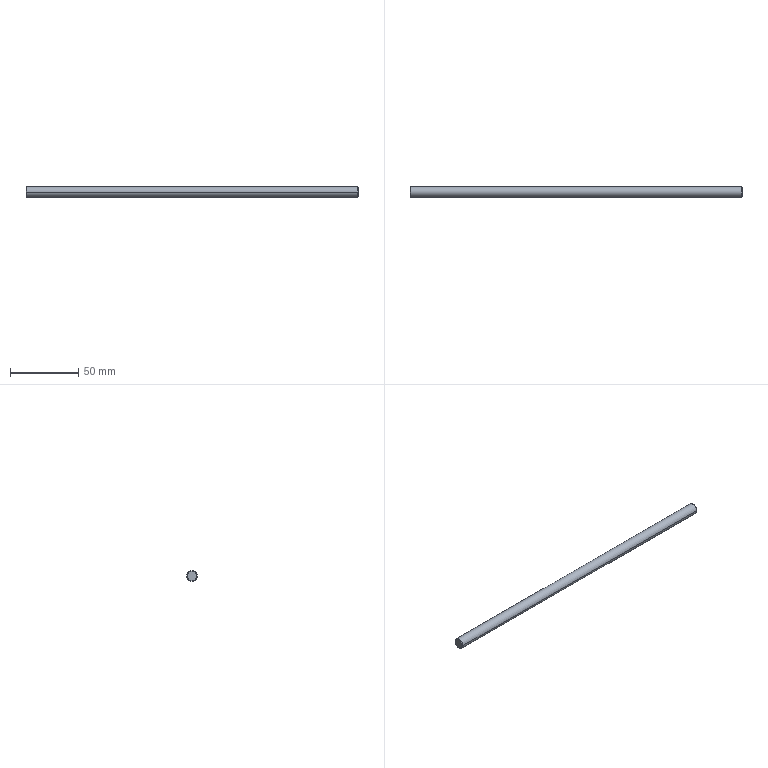Part | STEP file | 02-20 Φ8 polished rod | 1 solid | 8 faces | box 244 x 8 x 8 mm | volume 12259 mm3 | cone 4 | cylinder 2 | plane 2 | commonest cylinder face diameters 8 x2
STEP:
#1=CARTESIAN_POINT('',(0.,0.,0.));
#2=DIRECTION('',(0.,0.,1.));
#3=DIRECTION('',(1.,0.,0.));
#4=AXIS2_PLACEMENT_3D('',#1,#2,#3);
#5=CARTESIAN_POINT('',(-122.,0.,3.5));
#6=VERTEX_POINT('',#5);
#7=CARTESIAN_POINT('',(-122.,0.,-3.5));
#8=VERTEX_POINT('',#7);
#9=CARTESIAN_POINT('',(-122.,0.,0.));
#10=DIRECTION('',(-1.,0.,0.));
#11=DIRECTION('',(0.,0.,-1.));
#12=AXIS2_PLACEMENT_3D('',#9,#10,#11);
#13=CIRCLE('',#12,3.5);
#14=CARTESIAN_POINT('',(-122.,0.,0.));
#15=DIRECTION('',(1.,0.,0.));
#16=DIRECTION('',(0.,0.,-1.));
#17=AXIS2_PLACEMENT_3D('',#14,#15,#16);
#18=CONICAL_SURFACE('',#17,3.5,0.7854);
#19=CARTESIAN_POINT('',(6.283,0.));
#20=DIRECTION('',(-1.,0.));
#21=VECTOR('',#20,1.);
#22=LINE('',#19,#21);
#23=(GEOMETRIC_REPRESENTATION_CONTEXT(2)PARAMETRIC_REPRESENTATION_CONTEXT()REPRESENTATION_CONTEXT('',''));
#24=DEFINITIONAL_REPRESENTATION('',(#22),#23);
#25=PCURVE('',#18,#24);
#26=CARTESIAN_POINT('',(-122.,-3.542,3.542));
#27=DIRECTION('',(1.,0.,0.));
#28=DIRECTION('',(0.,0.,-1.));
#29=AXIS2_PLACEMENT_3D('',#26,#27,#28);
#30=PLANE('',#29);
#31=CARTESIAN_POINT('',(7.042,3.542));
#32=CARTESIAN_POINT('',(7.042,-2.52));
#33=CARTESIAN_POINT('',(1.792,0.5109));
#34=CARTESIAN_POINT('',(-3.458,3.542));
#35=CARTESIAN_POINT('',(1.792,6.573));
#36=CARTESIAN_POINT('',(7.042,9.604));
#37=CARTESIAN_POINT('',(7.042,3.542));
#38=(BOUNDED_CURVE()B_SPLINE_CURVE(2,(#31,#32,#33,#34,#35,#36,#37),.UNSPECIFIED.,.T.,.F.)B_SPLINE_CURVE_WITH_KNOTS((1,2,2,2,2,1),(-2.094,0.,2.094,4.189,6.283,8.378),.UNSPECIFIED.)CURVE()GEOMETRIC_REPRESENTATION_ITEM()RATIONAL_B_SPLINE_CURVE((1.,0.5,1.,0.5,1.,0.5,1.))REPRESENTATION_ITEM(''));
#39=(GEOMETRIC_REPRESENTATION_CONTEXT(2)PARAMETRIC_REPRESENTATION_CONTEXT()REPRESENTATION_CONTEXT('',''));
#40=DEFINITIONAL_REPRESENTATION('',(#38),#39);
#41=PCURVE('',#30,#40);
#42=SURFACE_CURVE('',#13,(#25,#41),.PCURVE_S1.);
#43=EDGE_CURVE('',#6,#8,#42,.T.);
#44=ORIENTED_EDGE('',*,*,#43,.F.);
#45=CARTESIAN_POINT('',(-121.5,0.,4.));
#46=VERTEX_POINT('',#45);
#47=CARTESIAN_POINT('',(-122.,0.,3.5));
#48=DIRECTION('',(0.7071,0.,0.7071));
#49=VECTOR('',#48,1.);
#50=LINE('',#47,#49);
#51=CARTESIAN_POINT('',(3.142,0.));
#52=DIRECTION('',(0.,1.));
#53=VECTOR('',#52,1.);
#54=LINE('',#51,#53);
#55=(GEOMETRIC_REPRESENTATION_CONTEXT(2)PARAMETRIC_REPRESENTATION_CONTEXT()REPRESENTATION_CONTEXT('',''));
#56=DEFINITIONAL_REPRESENTATION('',(#54),#55);
#57=PCURVE('',#18,#56);
#58=CARTESIAN_POINT('',(-122.,0.,0.));
#59=DIRECTION('',(1.,0.,0.));
#60=DIRECTION('',(0.,0.,-1.));
#61=AXIS2_PLACEMENT_3D('',#58,#59,#60);
#62=CONICAL_SURFACE('',#61,3.5,0.7854);
#63=CARTESIAN_POINT('',(3.142,0.));
#64=DIRECTION('',(0.,1.));
#65=VECTOR('',#64,1.);
#66=LINE('',#63,#65);
#67=(GEOMETRIC_REPRESENTATION_CONTEXT(2)PARAMETRIC_REPRESENTATION_CONTEXT()REPRESENTATION_CONTEXT('',''));
#68=DEFINITIONAL_REPRESENTATION('',(#66),#67);
#69=PCURVE('',#62,#68);
#70=SURFACE_CURVE('',#50,(#57,#69),.PCURVE_S1.);
#71=EDGE_CURVE('',#6,#46,#70,.T.);
#72=ORIENTED_EDGE('',*,*,#71,.T.);
#73=CARTESIAN_POINT('',(-121.5,4.,0.));
#74=VERTEX_POINT('',#73);
#75=CARTESIAN_POINT('',(-121.5,0.,0.));
#76=DIRECTION('',(1.,0.,0.));
#77=DIRECTION('',(0.,0.,-1.));
#78=AXIS2_PLACEMENT_3D('',#75,#76,#77);
#79=CIRCLE('',#78,4.);
#80=CARTESIAN_POINT('',(0.,0.5));
#81=DIRECTION('',(1.,0.));
#82=VECTOR('',#81,1.);
#83=LINE('',#80,#82);
#84=(GEOMETRIC_REPRESENTATION_CONTEXT(2)PARAMETRIC_REPRESENTATION_CONTEXT()REPRESENTATION_CONTEXT('',''));
#85=DEFINITIONAL_REPRESENTATION('',(#83),#84);
#86=PCURVE('',#18,#85);
#87=CARTESIAN_POINT('',(121.5,0.,0.));
#88=DIRECTION('',(-1.,0.,0.));
#89=DIRECTION('',(0.,-1.,0.));
#90=AXIS2_PLACEMENT_3D('',#87,#88,#89);
#91=CYLINDRICAL_SURFACE('',#90,4.);
#92=CARTESIAN_POINT('',(4.712,243.));
#93=DIRECTION('',(-1.,0.));
#94=VECTOR('',#93,1.);
#95=LINE('',#92,#94);
#96=(GEOMETRIC_REPRESENTATION_CONTEXT(2)PARAMETRIC_REPRESENTATION_CONTEXT()REPRESENTATION_CONTEXT('',''));
#97=DEFINITIONAL_REPRESENTATION('',(#95),#96);
#98=PCURVE('',#91,#97);
#99=SURFACE_CURVE('',#79,(#86,#98),.PCURVE_S1.);
#100=EDGE_CURVE('',#74,#46,#99,.T.);
#101=ORIENTED_EDGE('',*,*,#100,.F.);
#102=CARTESIAN_POINT('',(-121.5,0.,-4.));
#103=VERTEX_POINT('',#102);
#104=CARTESIAN_POINT('',(-121.5,0.,0.));
#105=DIRECTION('',(1.,0.,0.));
#106=DIRECTION('',(0.,0.,-1.));
#107=AXIS2_PLACEMENT_3D('',#104,#105,#106);
#108=CIRCLE('',#107,4.);
#109=CARTESIAN_POINT('',(0.,0.5));
#110=DIRECTION('',(1.,0.));
#111=VECTOR('',#110,1.);
#112=LINE('',#109,#111);
#113=(GEOMETRIC_REPRESENTATION_CONTEXT(2)PARAMETRIC_REPRESENTATION_CONTEXT()REPRESENTATION_CONTEXT('',''));
#114=DEFINITIONAL_REPRESENTATION('',(#112),#113);
#115=PCURVE('',#18,#114);
#116=CARTESIAN_POINT('',(121.5,0.,0.));
#117=DIRECTION('',(-1.,0.,0.));
#118=DIRECTION('',(0.,-1.,0.));
#119=AXIS2_PLACEMENT_3D('',#116,#117,#118);
#120=CYLINDRICAL_SURFACE('',#119,4.);
#121=CARTESIAN_POINT('',(4.712,243.));
#122=DIRECTION('',(-1.,0.));
#123=VECTOR('',#122,1.);
#124=LINE('',#121,#123);
#125=(GEOMETRIC_REPRESENTATION_CONTEXT(2)PARAMETRIC_REPRESENTATION_CONTEXT()REPRESENTATION_CONTEXT('',''));
#126=DEFINITIONAL_REPRESENTATION('',(#124),#125);
#127=PCURVE('',#120,#126);
#128=SURFACE_CURVE('',#108,(#115,#127),.PCURVE_S1.);
#129=EDGE_CURVE('',#103,#74,#128,.T.);
#130=ORIENTED_EDGE('',*,*,#129,.F.);
#131=CARTESIAN_POINT('',(-122.,0.,-3.5));
#132=DIRECTION('',(0.7071,0.,-0.7071));
#133=VECTOR('',#132,1.);
#134=LINE('',#131,#133);
#135=CARTESIAN_POINT('',(0.,0.));
#136=DIRECTION('',(0.,1.));
#137=VECTOR('',#136,1.);
#138=LINE('',#135,#137);
#139=(GEOMETRIC_REPRESENTATION_CONTEXT(2)PARAMETRIC_REPRESENTATION_CONTEXT()REPRESENTATION_CONTEXT('',''));
#140=DEFINITIONAL_REPRESENTATION('',(#138),#139);
#141=PCURVE('',#18,#140);
#142=CARTESIAN_POINT('',(6.283,0.));
#143=DIRECTION('',(0.,1.));
#144=VECTOR('',#143,1.);
#145=LINE('',#142,#144);
#146=(GEOMETRIC_REPRESENTATION_CONTEXT(2)PARAMETRIC_REPRESENTATION_CONTEXT()REPRESENTATION_CONTEXT('',''));
#147=DEFINITIONAL_REPRESENTATION('',(#145),#146);
#148=PCURVE('',#62,#147);
#149=SURFACE_CURVE('',#134,(#141,#148),.PCURVE_S1.);
#150=EDGE_CURVE('',#8,#103,#149,.T.);
#151=ORIENTED_EDGE('',*,*,#150,.F.);
#152=EDGE_LOOP('',(#44,#72,#101,#130,#151));
#153=FACE_BOUND('',#152,.T.);
#154=ADVANCED_FACE('',(#153),#18,.T.);
#155=CARTESIAN_POINT('',(121.5,4.,0.));
#156=VERTEX_POINT('',#155);
#157=CARTESIAN_POINT('',(121.5,0.,4.));
#158=VERTEX_POINT('',#157);
#159=CARTESIAN_POINT('',(121.5,0.,0.));
#160=DIRECTION('',(1.,0.,0.));
#161=DIRECTION('',(0.,0.,1.));
#162=AXIS2_PLACEMENT_3D('',#159,#160,#161);
#163=CIRCLE('',#162,4.);
#164=CARTESIAN_POINT('',(7.854,0.));
#165=DIRECTION('',(-1.,0.));
#166=VECTOR('',#165,1.);
#167=LINE('',#164,#166);
#168=(GEOMETRIC_REPRESENTATION_CONTEXT(2)PARAMETRIC_REPRESENTATION_CONTEXT()REPRESENTATION_CONTEXT('',''));
#169=DEFINITIONAL_REPRESENTATION('',(#167),#168);
#170=PCURVE('',#91,#169);
#171=CARTESIAN_POINT('',(122.,0.,0.));
#172=DIRECTION('',(-1.,0.,0.));
#173=DIRECTION('',(0.,0.,1.));
#174=AXIS2_PLACEMENT_3D('',#171,#172,#173);
#175=CONICAL_SURFACE('',#174,3.5,0.7854);
#176=CARTESIAN_POINT('',(6.283,0.5));
#177=DIRECTION('',(-1.,0.));
#178=VECTOR('',#177,1.);
#179=LINE('',#176,#178);
#180=(GEOMETRIC_REPRESENTATION_CONTEXT(2)PARAMETRIC_REPRESENTATION_CONTEXT()REPRESENTATION_CONTEXT('',''));
#181=DEFINITIONAL_REPRESENTATION('',(#179),#180);
#182=PCURVE('',#175,#181);
#183=SURFACE_CURVE('',#163,(#170,#182),.PCURVE_S1.);
#184=EDGE_CURVE('',#156,#158,#183,.T.);
#185=ORIENTED_EDGE('',*,*,#184,.F.);
#186=CARTESIAN_POINT('',(121.5,4.,0.));
#187=DIRECTION('',(-1.,0.,0.));
#188=VECTOR('',#187,1.);
#189=LINE('',#186,#188);
#190=CARTESIAN_POINT('',(3.142,0.));
#191=DIRECTION('',(0.,1.));
#192=VECTOR('',#191,1.);
#193=LINE('',#190,#192);
#194=(GEOMETRIC_REPRESENTATION_CONTEXT(2)PARAMETRIC_REPRESENTATION_CONTEXT()REPRESENTATION_CONTEXT('',''));
#195=DEFINITIONAL_REPRESENTATION('',(#193),#194);
#196=PCURVE('',#91,#195);
#197=CARTESIAN_POINT('',(3.142,0.));
#198=DIRECTION('',(0.,1.));
#199=VECTOR('',#198,1.);
#200=LINE('',#197,#199);
#201=(GEOMETRIC_REPRESENTATION_CONTEXT(2)PARAMETRIC_REPRESENTATION_CONTEXT()REPRESENTATION_CONTEXT('',''));
#202=DEFINITIONAL_REPRESENTATION('',(#200),#201);
#203=PCURVE('',#120,#202);
#204=SURFACE_CURVE('',#189,(#196,#203),.PCURVE_S1.);
#205=EDGE_CURVE('',#156,#74,#204,.T.);
#206=ORIENTED_EDGE('',*,*,#205,.T.);
#207=ORIENTED_EDGE('',*,*,#100,.T.);
#208=CARTESIAN_POINT('',(-121.5,-4.,0.));
#209=VERTEX_POINT('',#208);
#210=CARTESIAN_POINT('',(-121.5,0.,0.));
#211=DIRECTION('',(1.,0.,0.));
#212=DIRECTION('',(0.,0.,-1.));
#213=AXIS2_PLACEMENT_3D('',#210,#211,#212);
#214=CIRCLE('',#213,4.);
#215=CARTESIAN_POINT('',(4.712,243.));
#216=DIRECTION('',(-1.,0.));
#217=VECTOR('',#216,1.);
#218=LINE('',#215,#217);
#219=(GEOMETRIC_REPRESENTATION_CONTEXT(2)PARAMETRIC_REPRESENTATION_CONTEXT()REPRESENTATION_CONTEXT('',''));
#220=DEFINITIONAL_REPRESENTATION('',(#218),#219);
#221=PCURVE('',#91,#220);
#222=CARTESIAN_POINT('',(0.,0.5));
#223=DIRECTION('',(1.,0.));
#224=VECTOR('',#223,1.);
#225=LINE('',#222,#224);
#226=(GEOMETRIC_REPRESENTATION_CONTEXT(2)PARAMETRIC_REPRESENTATION_CONTEXT()REPRESENTATION_CONTEXT('',''));
#227=DEFINITIONAL_REPRESENTATION('',(#225),#226);
#228=PCURVE('',#62,#227);
#229=SURFACE_CURVE('',#214,(#221,#228),.PCURVE_S1.);
#230=EDGE_CURVE('',#46,#209,#229,.T.);
#231=ORIENTED_EDGE('',*,*,#230,.T.);
#232=CARTESIAN_POINT('',(121.5,-4.,0.));
#233=VERTEX_POINT('',#232);
#234=CARTESIAN_POINT('',(121.5,-4.,0.));
#235=DIRECTION('',(-1.,0.,0.));
#236=VECTOR('',#235,1.);
#237=LINE('',#234,#236);
#238=CARTESIAN_POINT('',(0.,0.));
#239=DIRECTION('',(0.,1.));
#240=VECTOR('',#239,1.);
#241=LINE('',#238,#240);
#242=(GEOMETRIC_REPRESENTATION_CONTEXT(2)PARAMETRIC_REPRESENTATION_CONTEXT()REPRESENTATION_CONTEXT('',''));
#243=DEFINITIONAL_REPRESENTATION('',(#241),#242);
#244=PCURVE('',#91,#243);
#245=CARTESIAN_POINT('',(6.283,0.));
#246=DIRECTION('',(0.,1.));
#247=VECTOR('',#246,1.);
#248=LINE('',#245,#247);
#249=(GEOMETRIC_REPRESENTATION_CONTEXT(2)PARAMETRIC_REPRESENTATION_CONTEXT()REPRESENTATION_CONTEXT('',''));
#250=DEFINITIONAL_REPRESENTATION('',(#248),#249);
#251=PCURVE('',#120,#250);
#252=SURFACE_CURVE('',#237,(#244,#251),.PCURVE_S1.);
#253=EDGE_CURVE('',#233,#209,#252,.T.);
#254=ORIENTED_EDGE('',*,*,#253,.F.);
#255=CARTESIAN_POINT('',(121.5,0.,0.));
#256=DIRECTION('',(1.,0.,0.));
#257=DIRECTION('',(0.,0.,1.));
#258=AXIS2_PLACEMENT_3D('',#255,#256,#257);
#259=CIRCLE('',#258,4.);
#260=CARTESIAN_POINT('',(1.571,0.));
#261=DIRECTION('',(-1.,0.));
#262=VECTOR('',#261,1.);
#263=LINE('',#260,#262);
#264=(GEOMETRIC_REPRESENTATION_CONTEXT(2)PARAMETRIC_REPRESENTATION_CONTEXT()REPRESENTATION_CONTEXT('',''));
#265=DEFINITIONAL_REPRESENTATION('',(#263),#264);
#266=PCURVE('',#91,#265);
#267=CARTESIAN_POINT('',(122.,0.,0.));
#268=DIRECTION('',(-1.,0.,0.));
#269=DIRECTION('',(0.,0.,1.));
#270=AXIS2_PLACEMENT_3D('',#267,#268,#269);
#271=CONICAL_SURFACE('',#270,3.5,0.7854);
#272=CARTESIAN_POINT('',(6.283,0.5));
#273=DIRECTION('',(-1.,0.));
#274=VECTOR('',#273,1.);
#275=LINE('',#272,#274);
#276=(GEOMETRIC_REPRESENTATION_CONTEXT(2)PARAMETRIC_REPRESENTATION_CONTEXT()REPRESENTATION_CONTEXT('',''));
#277=DEFINITIONAL_REPRESENTATION('',(#275),#276);
#278=PCURVE('',#271,#277);
#279=SURFACE_CURVE('',#259,(#266,#278),.PCURVE_S1.);
#280=EDGE_CURVE('',#158,#233,#279,.T.);
#281=ORIENTED_EDGE('',*,*,#280,.F.);
#282=EDGE_LOOP('',(#185,#206,#207,#231,#254,#281));
#283=FACE_BOUND('',#282,.T.);
#284=ADVANCED_FACE('',(#283),#91,.T.);
#285=CARTESIAN_POINT('',(122.,0.,-3.5));
#286=VERTEX_POINT('',#285);
#287=CARTESIAN_POINT('',(122.,0.,3.5));
#288=VERTEX_POINT('',#287);
#289=CARTESIAN_POINT('',(122.,0.,0.));
#290=DIRECTION('',(1.,0.,0.));
#291=DIRECTION('',(0.,0.,1.));
#292=AXIS2_PLACEMENT_3D('',#289,#290,#291);
#293=CIRCLE('',#292,3.5);
#294=CARTESIAN_POINT('',(6.283,0.));
#295=DIRECTION('',(-1.,0.));
#296=VECTOR('',#295,1.);
#297=LINE('',#294,#296);
#298=(GEOMETRIC_REPRESENTATION_CONTEXT(2)PARAMETRIC_REPRESENTATION_CONTEXT()REPRESENTATION_CONTEXT('',''));
#299=DEFINITIONAL_REPRESENTATION('',(#297),#298);
#300=PCURVE('',#175,#299);
#301=CARTESIAN_POINT('',(122.,-3.542,3.542));
#302=DIRECTION('',(1.,0.,0.));
#303=DIRECTION('',(0.,0.,-1.));
#304=AXIS2_PLACEMENT_3D('',#301,#302,#303);
#305=PLANE('',#304);
#306=CARTESIAN_POINT('',(3.542,3.542));
#307=DIRECTION('',(-1.,0.));
#308=AXIS2_PLACEMENT_2D('',#306,#307);
#309=CIRCLE('',#308,3.5);
#310=(GEOMETRIC_REPRESENTATION_CONTEXT(2)PARAMETRIC_REPRESENTATION_CONTEXT()REPRESENTATION_CONTEXT('',''));
#311=DEFINITIONAL_REPRESENTATION('',(#309),#310);
#312=PCURVE('',#305,#311);
#313=SURFACE_CURVE('',#293,(#300,#312),.PCURVE_S1.);
#314=EDGE_CURVE('',#286,#288,#313,.T.);
#315=ORIENTED_EDGE('',*,*,#314,.F.);
#316=CARTESIAN_POINT('',(121.5,0.,-4.));
#317=VERTEX_POINT('',#316);
#318=CARTESIAN_POINT('',(122.,0.,-3.5));
#319=DIRECTION('',(-0.7071,0.,-0.7071));
#320=VECTOR('',#319,1.);
#321=LINE('',#318,#320);
#322=CARTESIAN_POINT('',(3.142,0.));
#323=DIRECTION('',(0.,1.));
#324=VECTOR('',#323,1.);
#325=LINE('',#322,#324);
#326=(GEOMETRIC_REPRESENTATION_CONTEXT(2)PARAMETRIC_REPRESENTATION_CONTEXT()REPRESENTATION_CONTEXT('',''));
#327=DEFINITIONAL_REPRESENTATION('',(#325),#326);
#328=PCURVE('',#175,#327);
#329=CARTESIAN_POINT('',(3.142,0.));
#330=DIRECTION('',(0.,1.));
#331=VECTOR('',#330,1.);
#332=LINE('',#329,#331);
#333=(GEOMETRIC_REPRESENTATION_CONTEXT(2)PARAMETRIC_REPRESENTATION_CONTEXT()REPRESENTATION_CONTEXT('',''));
#334=DEFINITIONAL_REPRESENTATION('',(#332),#333);
#335=PCURVE('',#271,#334);
#336=SURFACE_CURVE('',#321,(#328,#335),.PCURVE_S1.);
#337=EDGE_CURVE('',#286,#317,#336,.T.);
#338=ORIENTED_EDGE('',*,*,#337,.T.);
#339=CARTESIAN_POINT('',(121.5,0.,0.));
#340=DIRECTION('',(1.,0.,0.));
#341=DIRECTION('',(0.,0.,1.));
#342=AXIS2_PLACEMENT_3D('',#339,#340,#341);
#343=CIRCLE('',#342,4.);
#344=CARTESIAN_POINT('',(6.283,0.5));
#345=DIRECTION('',(-1.,0.));
#346=VECTOR('',#345,1.);
#347=LINE('',#344,#346);
#348=(GEOMETRIC_REPRESENTATION_CONTEXT(2)PARAMETRIC_REPRESENTATION_CONTEXT()REPRESENTATION_CONTEXT('',''));
#349=DEFINITIONAL_REPRESENTATION('',(#347),#348);
#350=PCURVE('',#175,#349);
#351=CARTESIAN_POINT('',(7.854,0.));
#352=DIRECTION('',(-1.,0.));
#353=VECTOR('',#352,1.);
#354=LINE('',#351,#353);
#355=(GEOMETRIC_REPRESENTATION_CONTEXT(2)PARAMETRIC_REPRESENTATION_CONTEXT()REPRESENTATION_CONTEXT('',''));
#356=DEFINITIONAL_REPRESENTATION('',(#354),#355);
#357=PCURVE('',#120,#356);
#358=SURFACE_CURVE('',#343,(#350,#357),.PCURVE_S1.);
#359=EDGE_CURVE('',#317,#156,#358,.T.);
#360=ORIENTED_EDGE('',*,*,#359,.T.);
#361=ORIENTED_EDGE('',*,*,#184,.T.);
#362=CARTESIAN_POINT('',(122.,0.,3.5));
#363=DIRECTION('',(-0.7071,0.,0.7071));
#364=VECTOR('',#363,1.);
#365=LINE('',#362,#364);
#366=CARTESIAN_POINT('',(0.,0.));
#367=DIRECTION('',(0.,1.));
#368=VECTOR('',#367,1.);
#369=LINE('',#366,#368);
#370=(GEOMETRIC_REPRESENTATION_CONTEXT(2)PARAMETRIC_REPRESENTATION_CONTEXT()REPRESENTATION_CONTEXT('',''));
#371=DEFINITIONAL_REPRESENTATION('',(#369),#370);
#372=PCURVE('',#175,#371);
#373=CARTESIAN_POINT('',(6.283,0.));
#374=DIRECTION('',(0.,1.));
#375=VECTOR('',#374,1.);
#376=LINE('',#373,#375);
#377=(GEOMETRIC_REPRESENTATION_CONTEXT(2)PARAMETRIC_REPRESENTATION_CONTEXT()REPRESENTATION_CONTEXT('',''));
#378=DEFINITIONAL_REPRESENTATION('',(#376),#377);
#379=PCURVE('',#271,#378);
#380=SURFACE_CURVE('',#365,(#372,#379),.PCURVE_S1.);
#381=EDGE_CURVE('',#288,#158,#380,.T.);
#382=ORIENTED_EDGE('',*,*,#381,.F.);
#383=EDGE_LOOP('',(#315,#338,#360,#361,#382));
#384=FACE_BOUND('',#383,.T.);
#385=ADVANCED_FACE('',(#384),#175,.T.);
#386=ORIENTED_EDGE('',*,*,#71,.F.);
#387=CARTESIAN_POINT('',(-122.,0.,0.));
#388=DIRECTION('',(-1.,0.,0.));
#389=DIRECTION('',(0.,0.,-1.));
#390=AXIS2_PLACEMENT_3D('',#387,#388,#389);
#391=CIRCLE('',#390,3.5);
#392=CARTESIAN_POINT('',(6.283,0.));
#393=DIRECTION('',(-1.,0.));
#394=VECTOR('',#393,1.);
#395=LINE('',#392,#394);
#396=(GEOMETRIC_REPRESENTATION_CONTEXT(2)PARAMETRIC_REPRESENTATION_CONTEXT()REPRESENTATION_CONTEXT('',''));
#397=DEFINITIONAL_REPRESENTATION('',(#395),#396);
#398=PCURVE('',#62,#397);
#399=CARTESIAN_POINT('',(7.042,3.542));
#400=CARTESIAN_POINT('',(7.042,-2.52));
#401=CARTESIAN_POINT('',(1.792,0.5109));
#402=CARTESIAN_POINT('',(-3.458,3.542));
#403=CARTESIAN_POINT('',(1.792,6.573));
#404=CARTESIAN_POINT('',(7.042,9.604));
#405=CARTESIAN_POINT('',(7.042,3.542));
#406=(BOUNDED_CURVE()B_SPLINE_CURVE(2,(#399,#400,#401,#402,#403,#404,#405),.UNSPECIFIED.,.T.,.F.)B_SPLINE_CURVE_WITH_KNOTS((1,2,2,2,2,1),(-2.094,0.,2.094,4.189,6.283,8.378),.UNSPECIFIED.)CURVE()GEOMETRIC_REPRESENTATION_ITEM()RATIONAL_B_SPLINE_CURVE((1.,0.5,1.,0.5,1.,0.5,1.))REPRESENTATION_ITEM(''));
#407=(GEOMETRIC_REPRESENTATION_CONTEXT(2)PARAMETRIC_REPRESENTATION_CONTEXT()REPRESENTATION_CONTEXT('',''));
#408=DEFINITIONAL_REPRESENTATION('',(#406),#407);
#409=PCURVE('',#30,#408);
#410=SURFACE_CURVE('',#391,(#398,#409),.PCURVE_S1.);
#411=EDGE_CURVE('',#8,#6,#410,.T.);
#412=ORIENTED_EDGE('',*,*,#411,.F.);
#413=ORIENTED_EDGE('',*,*,#150,.T.);
#414=CARTESIAN_POINT('',(-121.5,0.,0.));
#415=DIRECTION('',(1.,0.,0.));
#416=DIRECTION('',(0.,0.,-1.));
#417=AXIS2_PLACEMENT_3D('',#414,#415,#416);
#418=CIRCLE('',#417,4.);
#419=CARTESIAN_POINT('',(0.,0.5));
#420=DIRECTION('',(1.,0.));
#421=VECTOR('',#420,1.);
#422=LINE('',#419,#421);
#423=(GEOMETRIC_REPRESENTATION_CONTEXT(2)PARAMETRIC_REPRESENTATION_CONTEXT()REPRESENTATION_CONTEXT('',''));
#424=DEFINITIONAL_REPRESENTATION('',(#422),#423);
#425=PCURVE('',#62,#424);
#426=CARTESIAN_POINT('',(10.996,243.));
#427=DIRECTION('',(-1.,0.));
#428=VECTOR('',#427,1.);
#429=LINE('',#426,#428);
#430=(GEOMETRIC_REPRESENTATION_CONTEXT(2)PARAMETRIC_REPRESENTATION_CONTEXT()REPRESENTATION_CONTEXT('',''));
#431=DEFINITIONAL_REPRESENTATION('',(#429),#430);
#432=PCURVE('',#120,#431);
#433=SURFACE_CURVE('',#418,(#425,#432),.PCURVE_S1.);
#434=EDGE_CURVE('',#209,#103,#433,.T.);
#435=ORIENTED_EDGE('',*,*,#434,.F.);
#436=ORIENTED_EDGE('',*,*,#230,.F.);
#437=EDGE_LOOP('',(#386,#412,#413,#435,#436));
#438=FACE_BOUND('',#437,.T.);
#439=ADVANCED_FACE('',(#438),#62,.T.);
#440=ORIENTED_EDGE('',*,*,#411,.T.);
#441=ORIENTED_EDGE('',*,*,#43,.T.);
#442=EDGE_LOOP('',(#440,#441));
#443=FACE_BOUND('',#442,.T.);
#444=ADVANCED_FACE('',(#443),#30,.F.);
#445=ORIENTED_EDGE('',*,*,#205,.F.);
#446=ORIENTED_EDGE('',*,*,#359,.F.);
#447=CARTESIAN_POINT('',(121.5,0.,0.));
#448=DIRECTION('',(1.,0.,0.));
#449=DIRECTION('',(0.,0.,1.));
#450=AXIS2_PLACEMENT_3D('',#447,#448,#449);
#451=CIRCLE('',#450,4.);
#452=CARTESIAN_POINT('',(7.854,0.));
#453=DIRECTION('',(-1.,0.));
#454=VECTOR('',#453,1.);
#455=LINE('',#452,#454);
#456=(GEOMETRIC_REPRESENTATION_CONTEXT(2)PARAMETRIC_REPRESENTATION_CONTEXT()REPRESENTATION_CONTEXT('',''));
#457=DEFINITIONAL_REPRESENTATION('',(#455),#456);
#458=PCURVE('',#120,#457);
#459=CARTESIAN_POINT('',(6.283,0.5));
#460=DIRECTION('',(-1.,0.));
#461=VECTOR('',#460,1.);
#462=LINE('',#459,#461);
#463=(GEOMETRIC_REPRESENTATION_CONTEXT(2)PARAMETRIC_REPRESENTATION_CONTEXT()REPRESENTATION_CONTEXT('',''));
#464=DEFINITIONAL_REPRESENTATION('',(#462),#463);
#465=PCURVE('',#271,#464);
#466=SURFACE_CURVE('',#451,(#458,#465),.PCURVE_S1.);
#467=EDGE_CURVE('',#233,#317,#466,.T.);
#468=ORIENTED_EDGE('',*,*,#467,.F.);
#469=ORIENTED_EDGE('',*,*,#253,.T.);
#470=ORIENTED_EDGE('',*,*,#434,.T.);
#471=ORIENTED_EDGE('',*,*,#129,.T.);
#472=EDGE_LOOP('',(#445,#446,#468,#469,#470,#471));
#473=FACE_BOUND('',#472,.T.);
#474=ADVANCED_FACE('',(#473),#120,.T.);
#475=ORIENTED_EDGE('',*,*,#337,.F.);
#476=CARTESIAN_POINT('',(122.,0.,0.));
#477=DIRECTION('',(1.,0.,0.));
#478=DIRECTION('',(0.,0.,1.));
#479=AXIS2_PLACEMENT_3D('',#476,#477,#478);
#480=CIRCLE('',#479,3.5);
#481=CARTESIAN_POINT('',(6.283,0.));
#482=DIRECTION('',(-1.,0.));
#483=VECTOR('',#482,1.);
#484=LINE('',#481,#483);
#485=(GEOMETRIC_REPRESENTATION_CONTEXT(2)PARAMETRIC_REPRESENTATION_CONTEXT()REPRESENTATION_CONTEXT('',''));
#486=DEFINITIONAL_REPRESENTATION('',(#484),#485);
#487=PCURVE('',#271,#486);
#488=CARTESIAN_POINT('',(3.542,3.542));
#489=DIRECTION('',(-1.,0.));
#490=AXIS2_PLACEMENT_2D('',#488,#489);
#491=CIRCLE('',#490,3.5);
#492=(GEOMETRIC_REPRESENTATION_CONTEXT(2)PARAMETRIC_REPRESENTATION_CONTEXT()REPRESENTATION_CONTEXT('',''));
#493=DEFINITIONAL_REPRESENTATION('',(#491),#492);
#494=PCURVE('',#305,#493);
#495=SURFACE_CURVE('',#480,(#487,#494),.PCURVE_S1.);
#496=EDGE_CURVE('',#288,#286,#495,.T.);
#497=ORIENTED_EDGE('',*,*,#496,.F.);
#498=ORIENTED_EDGE('',*,*,#381,.T.);
#499=ORIENTED_EDGE('',*,*,#280,.T.);
#500=ORIENTED_EDGE('',*,*,#467,.T.);
#501=EDGE_LOOP('',(#475,#497,#498,#499,#500));
#502=FACE_BOUND('',#501,.T.);
#503=ADVANCED_FACE('',(#502),#271,.T.);
#504=ORIENTED_EDGE('',*,*,#496,.T.);
#505=ORIENTED_EDGE('',*,*,#314,.T.);
#506=EDGE_LOOP('',(#504,#505));
#507=FACE_BOUND('',#506,.T.);
#508=ADVANCED_FACE('',(#507),#305,.T.);
#509=CLOSED_SHELL('',(#154,#284,#385,#439,#444,#474,#503,#508));
#510=MANIFOLD_SOLID_BREP('',#509);
#511=(LENGTH_UNIT()NAMED_UNIT(*)SI_UNIT(.MILLI.,.METRE.));
#512=UNCERTAINTY_MEASURE_WITH_UNIT(LENGTH_MEASURE(0.0000001),#511,'','');
#513=(NAMED_UNIT(*)PLANE_ANGLE_UNIT()SI_UNIT($,.RADIAN.));
#514=(NAMED_UNIT(*)SI_UNIT($,.STERADIAN.)SOLID_ANGLE_UNIT());
#515=(GEOMETRIC_REPRESENTATION_CONTEXT(3)GLOBAL_UNCERTAINTY_ASSIGNED_CONTEXT((#512))GLOBAL_UNIT_ASSIGNED_CONTEXT((#511,#513,#514))REPRESENTATION_CONTEXT('',''));
#516=ADVANCED_BREP_SHAPE_REPRESENTATION('',(#4,#510),#515);